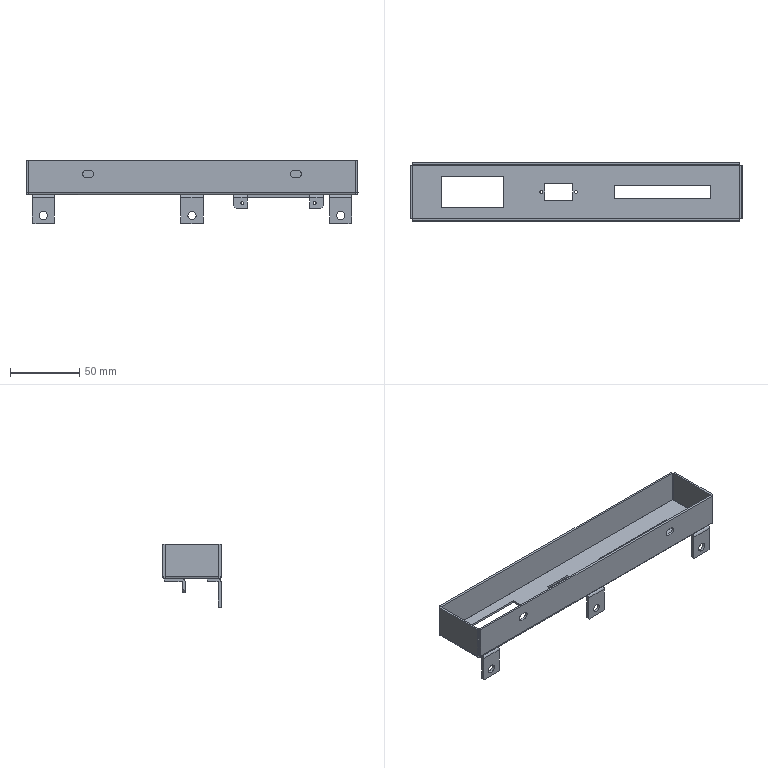Part | NX | features BREP 5 | 5 solids | 128 faces | box 240 x 42 x 46 mm | volume 35729 mm3 | plane 84 | cylinder 36 | spline 8 | commonest cylinder face diameters 6 x6 0.2 x5 4.2 x5 0.02 x4 2.05 x4 2.113 x4